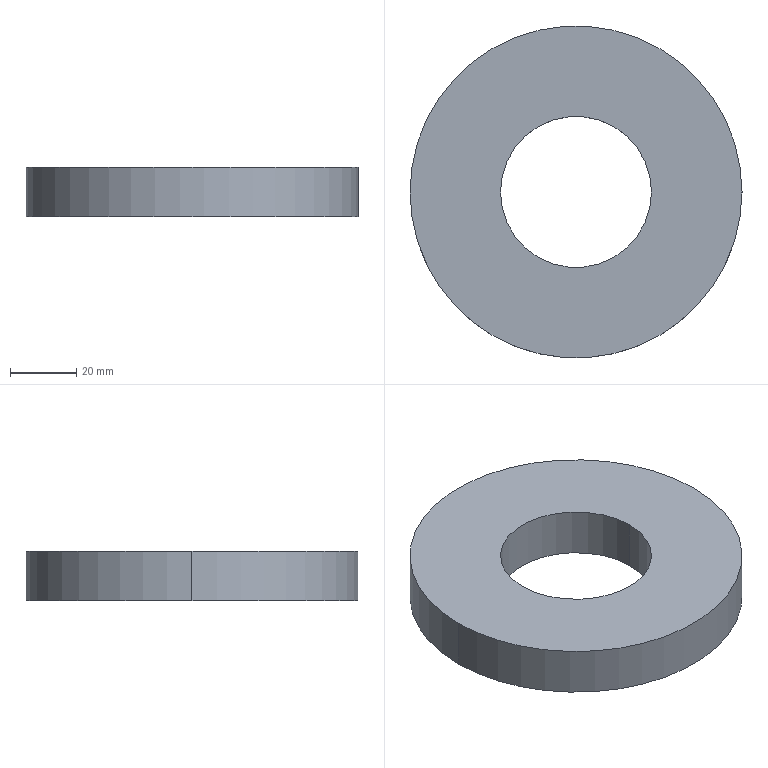Part | SolidWorks | features Extrusion 1 | 1 solid | 6 faces | box 100 x 100 x 15 mm | volume 93420 mm3 | cylinder 4 | plane 2 | commonest cylinder face diameters 45.5 x2 100 x2
STEP:
#1=CARTESIAN_POINT('',(-22.75,0.,15.));
#2=VERTEX_POINT('',#1);
#3=CARTESIAN_POINT('',(22.75,0.,15.));
#4=VERTEX_POINT('',#3);
#5=CARTESIAN_POINT('',(0.,0.,15.));
#6=DIRECTION('',(0.,0.,1.));
#7=DIRECTION('',(1.,0.,0.));
#8=AXIS2_PLACEMENT_3D('',#5,#6,#7);
#9=CIRCLE('',#8,22.75);
#10=EDGE_CURVE('',#2,#4,#9,.T.);
#11=ORIENTED_EDGE('',*,*,#10,.T.);
#12=CARTESIAN_POINT('',(22.75,0.,0.));
#13=VERTEX_POINT('',#12);
#14=CARTESIAN_POINT('',(22.75,0.,15.));
#15=DIRECTION('',(0.,0.,-1.));
#16=VECTOR('',#15,1000.);
#17=LINE('',#14,#16);
#18=EDGE_CURVE('',#4,#13,#17,.T.);
#19=ORIENTED_EDGE('',*,*,#18,.T.);
#20=CARTESIAN_POINT('',(-22.75,0.,0.));
#21=VERTEX_POINT('',#20);
#22=CARTESIAN_POINT('',(0.,0.,0.));
#23=DIRECTION('',(0.,0.,1.));
#24=DIRECTION('',(1.,0.,0.));
#25=AXIS2_PLACEMENT_3D('',#22,#23,#24);
#26=CIRCLE('',#25,22.75);
#27=EDGE_CURVE('',#21,#13,#26,.T.);
#28=ORIENTED_EDGE('',*,*,#27,.F.);
#29=CARTESIAN_POINT('',(-22.75,0.,15.));
#30=DIRECTION('',(0.,0.,-1.));
#31=VECTOR('',#30,1000.);
#32=LINE('',#29,#31);
#33=EDGE_CURVE('',#2,#21,#32,.T.);
#34=ORIENTED_EDGE('',*,*,#33,.F.);
#35=EDGE_LOOP('',(#11,#19,#28,#34));
#36=FACE_OUTER_BOUND('',#35,.T.);
#37=CARTESIAN_POINT('',(0.,0.,15.));
#38=DIRECTION('',(0.,0.,-1.));
#39=DIRECTION('',(-1.,0.,0.));
#40=AXIS2_PLACEMENT_3D('',#37,#38,#39);
#41=CYLINDRICAL_SURFACE('',#40,22.75);
#42=ADVANCED_FACE('',(#36),#41,.F.);
#43=CARTESIAN_POINT('',(50.,0.,15.));
#44=VERTEX_POINT('',#43);
#45=CARTESIAN_POINT('',(-50.,0.,15.));
#46=VERTEX_POINT('',#45);
#47=CARTESIAN_POINT('',(0.,0.,15.));
#48=DIRECTION('',(0.,0.,1.));
#49=DIRECTION('',(1.,0.,0.));
#50=AXIS2_PLACEMENT_3D('',#47,#48,#49);
#51=CIRCLE('',#50,50.);
#52=EDGE_CURVE('',#44,#46,#51,.T.);
#53=ORIENTED_EDGE('',*,*,#52,.F.);
#54=CARTESIAN_POINT('',(50.,0.,0.));
#55=VERTEX_POINT('',#54);
#56=CARTESIAN_POINT('',(50.,0.,15.));
#57=DIRECTION('',(0.,0.,-1.));
#58=VECTOR('',#57,1000.);
#59=LINE('',#56,#58);
#60=EDGE_CURVE('',#44,#55,#59,.T.);
#61=ORIENTED_EDGE('',*,*,#60,.T.);
#62=CARTESIAN_POINT('',(-50.,0.,0.));
#63=VERTEX_POINT('',#62);
#64=CARTESIAN_POINT('',(0.,0.,0.));
#65=DIRECTION('',(0.,0.,1.));
#66=DIRECTION('',(1.,0.,0.));
#67=AXIS2_PLACEMENT_3D('',#64,#65,#66);
#68=CIRCLE('',#67,50.);
#69=EDGE_CURVE('',#55,#63,#68,.T.);
#70=ORIENTED_EDGE('',*,*,#69,.T.);
#71=CARTESIAN_POINT('',(-50.,0.,15.));
#72=DIRECTION('',(0.,0.,-1.));
#73=VECTOR('',#72,1000.);
#74=LINE('',#71,#73);
#75=EDGE_CURVE('',#46,#63,#74,.T.);
#76=ORIENTED_EDGE('',*,*,#75,.F.);
#77=EDGE_LOOP('',(#53,#61,#70,#76));
#78=FACE_OUTER_BOUND('',#77,.T.);
#79=CARTESIAN_POINT('',(0.,0.,15.));
#80=DIRECTION('',(0.,0.,-1.));
#81=DIRECTION('',(-1.,0.,0.));
#82=AXIS2_PLACEMENT_3D('',#79,#80,#81);
#83=CYLINDRICAL_SURFACE('',#82,50.);
#84=ADVANCED_FACE('',(#78),#83,.T.);
#85=CARTESIAN_POINT('',(0.,0.,15.));
#86=DIRECTION('',(0.,0.,1.));
#87=DIRECTION('',(1.,0.,0.));
#88=AXIS2_PLACEMENT_3D('',#85,#86,#87);
#89=CIRCLE('',#88,50.);
#90=EDGE_CURVE('',#46,#44,#89,.T.);
#91=ORIENTED_EDGE('',*,*,#90,.T.);
#92=ORIENTED_EDGE('',*,*,#52,.T.);
#93=EDGE_LOOP('',(#91,#92));
#94=FACE_OUTER_BOUND('',#93,.T.);
#95=ORIENTED_EDGE('',*,*,#10,.F.);
#96=CARTESIAN_POINT('',(0.,0.,15.));
#97=DIRECTION('',(0.,0.,1.));
#98=DIRECTION('',(1.,0.,0.));
#99=AXIS2_PLACEMENT_3D('',#96,#97,#98);
#100=CIRCLE('',#99,22.75);
#101=EDGE_CURVE('',#4,#2,#100,.T.);
#102=ORIENTED_EDGE('',*,*,#101,.F.);
#103=EDGE_LOOP('',(#95,#102));
#104=FACE_BOUND('',#103,.T.);
#105=CARTESIAN_POINT('',(0.,0.,15.));
#106=DIRECTION('',(0.,0.,1.));
#107=DIRECTION('',(1.,0.,0.));
#108=AXIS2_PLACEMENT_3D('',#105,#106,#107);
#109=PLANE('',#108);
#110=ADVANCED_FACE('',(#94,#104),#109,.T.);
#111=CARTESIAN_POINT('',(0.,0.,0.));
#112=DIRECTION('',(0.,0.,1.));
#113=DIRECTION('',(1.,0.,0.));
#114=AXIS2_PLACEMENT_3D('',#111,#112,#113);
#115=CIRCLE('',#114,50.);
#116=EDGE_CURVE('',#63,#55,#115,.T.);
#117=ORIENTED_EDGE('',*,*,#116,.F.);
#118=ORIENTED_EDGE('',*,*,#69,.F.);
#119=EDGE_LOOP('',(#117,#118));
#120=FACE_OUTER_BOUND('',#119,.T.);
#121=ORIENTED_EDGE('',*,*,#27,.T.);
#122=CARTESIAN_POINT('',(0.,0.,0.));
#123=DIRECTION('',(0.,0.,1.));
#124=DIRECTION('',(1.,0.,0.));
#125=AXIS2_PLACEMENT_3D('',#122,#123,#124);
#126=CIRCLE('',#125,22.75);
#127=EDGE_CURVE('',#13,#21,#126,.T.);
#128=ORIENTED_EDGE('',*,*,#127,.T.);
#129=EDGE_LOOP('',(#121,#128));
#130=FACE_BOUND('',#129,.T.);
#131=CARTESIAN_POINT('',(0.,0.,0.));
#132=DIRECTION('',(0.,0.,1.));
#133=DIRECTION('',(1.,0.,0.));
#134=AXIS2_PLACEMENT_3D('',#131,#132,#133);
#135=PLANE('',#134);
#136=ADVANCED_FACE('',(#120,#130),#135,.F.);
#137=ORIENTED_EDGE('',*,*,#60,.F.);
#138=ORIENTED_EDGE('',*,*,#90,.F.);
#139=ORIENTED_EDGE('',*,*,#75,.T.);
#140=ORIENTED_EDGE('',*,*,#116,.T.);
#141=EDGE_LOOP('',(#137,#138,#139,#140));
#142=FACE_OUTER_BOUND('',#141,.T.);
#143=CARTESIAN_POINT('',(0.,0.,15.));
#144=DIRECTION('',(0.,0.,-1.));
#145=DIRECTION('',(-1.,0.,0.));
#146=AXIS2_PLACEMENT_3D('',#143,#144,#145);
#147=CYLINDRICAL_SURFACE('',#146,50.);
#148=ADVANCED_FACE('',(#142),#147,.T.);
#149=ORIENTED_EDGE('',*,*,#18,.F.);
#150=ORIENTED_EDGE('',*,*,#101,.T.);
#151=ORIENTED_EDGE('',*,*,#33,.T.);
#152=ORIENTED_EDGE('',*,*,#127,.F.);
#153=EDGE_LOOP('',(#149,#150,#151,#152));
#154=FACE_OUTER_BOUND('',#153,.T.);
#155=CARTESIAN_POINT('',(0.,0.,15.));
#156=DIRECTION('',(0.,0.,-1.));
#157=DIRECTION('',(-1.,0.,0.));
#158=AXIS2_PLACEMENT_3D('',#155,#156,#157);
#159=CYLINDRICAL_SURFACE('',#158,22.75);
#160=ADVANCED_FACE('',(#154),#159,.F.);
#161=CLOSED_SHELL('',(#42,#84,#110,#136,#148,#160));
#162=MANIFOLD_SOLID_BREP('',#161);
#163=CARTESIAN_POINT('',(0.,0.,0.));
#164=DIRECTION('',(0.,0.,1.));
#165=DIRECTION('',(1.,0.,0.));
#166=AXIS2_PLACEMENT_3D('',#163,#164,#165);
#167=(LENGTH_UNIT()NAMED_UNIT(*)SI_UNIT(.MILLI.,.METRE.));
#168=UNCERTAINTY_MEASURE_WITH_UNIT(LENGTH_MEASURE(0.00001),#167,'','');
#169=(NAMED_UNIT(*)PLANE_ANGLE_UNIT()SI_UNIT($,.RADIAN.));
#170=(NAMED_UNIT(*)SI_UNIT($,.STERADIAN.)SOLID_ANGLE_UNIT());
#171=(GEOMETRIC_REPRESENTATION_CONTEXT(3)GLOBAL_UNCERTAINTY_ASSIGNED_CONTEXT((#168))GLOBAL_UNIT_ASSIGNED_CONTEXT((#167,#169,#170))REPRESENTATION_CONTEXT('',''));
#172=ADVANCED_BREP_SHAPE_REPRESENTATION('',(#162,#166),#171);